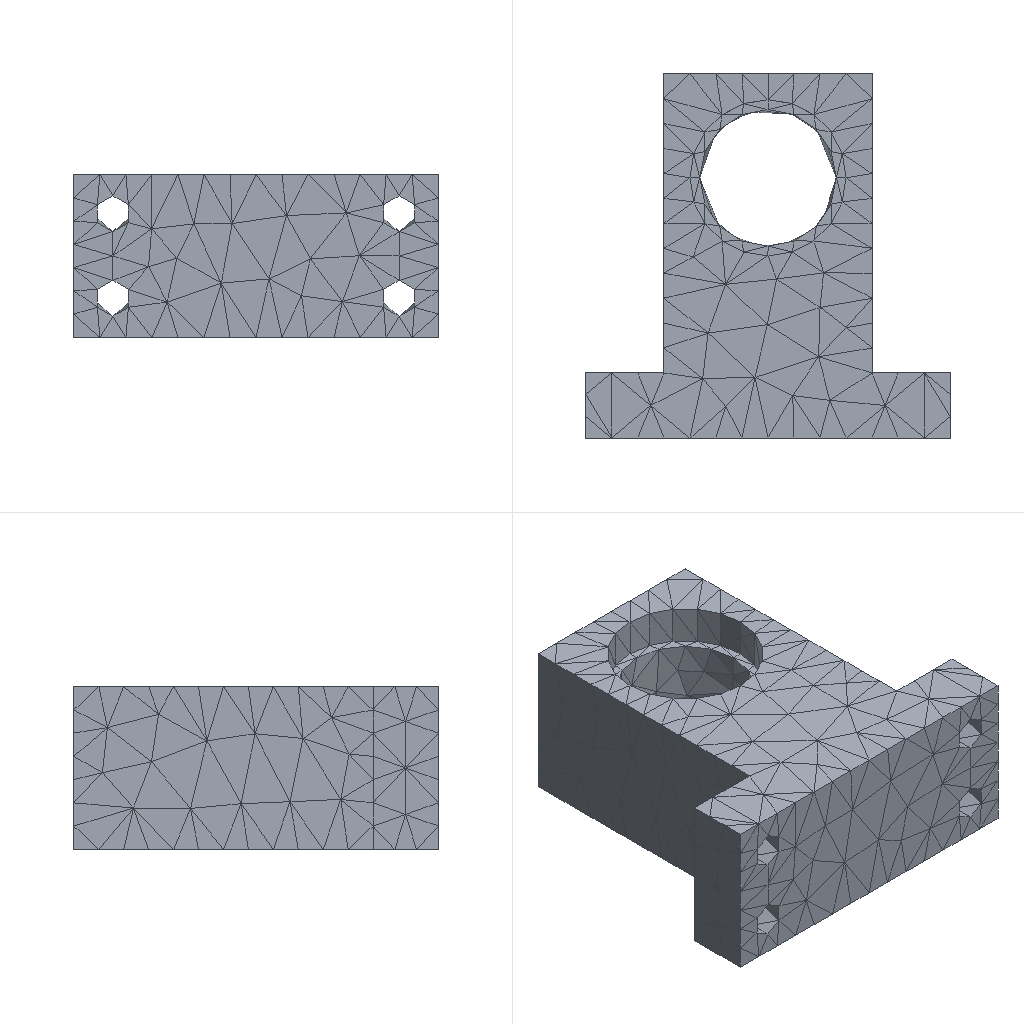Simulation study | ansys mapdl
Set-up summary:
category,name,step,type,value,unit,region
solver,ansys_mapdl
solver,version,,,22.1
units,MPA,,stated
analysis,deck,,static,static
load_step,requested,,,1
analysis,nlgeom,,,False
mesh,nodes,,,3282
mesh,elements,,,1777
element_type,ANSYS 187 (type 1),,solid,1667
element_type,ANSYS 154 (type 2),,surface,110
load,load commands in deck,,count,3
bc,support commands in deck,,count,1
named_set,_FIXEDSU,,component
material,1,,in results
check,setup vs results,,match,110 surface effect element(s) are not in the reader's mesh and were not compared
Ansys APDL input file, long lists of numbers shortened:
/batch
/config,noeldb,1     ! force off writing results to database
*get,_wallstrt,active,,time,wall
! ANSYS input file written by Workbench version 2022 R1
! File used for geometry attach: [REDACTED]
/title,wbnew--____ (A5)
! ****** Begin Custom Load Command Snippet ******
/COM, ACT Extensions:
/COM,     LSDYNA, 2021.1
/COM,
! ****** End   Custom Load Command Snippet ******
*DIM,_wb_ProjectScratch_dir,string,248
_wb_ProjectScratch_dir(1) = 'C:\Users\Administrator\AppData\Local\Temp\WB_Administrator_78380_2\_ProjectScratch\Scr73FA\'
*DIM,_wb_SolverFiles_dir,string,248
_wb_SolverFiles_dir(1) = 'C:\Users\Administrator\AppData\Local\Temp\WB_Administrator_78380_2\wbnew_files\dp0\SYS\MECH\'
*DIM,_wb_userfiles_dir,string,248
_wb_userfiles_dir(1) = 'C:\Users\Administrator\AppData\Local\Temp\WB_Administrator_78380_2\wbnew_files\user_files\'
/com,--- Data in consistent NMM units. See Solving Units in the help system for more information.
/units,MPA
/nopr
/wb,file,start              !  signify a WB generated input file
/prep7
! Turn off shape checking because checks already performed inside WB mesher.
! See help system for more information.
SHPP,OFF,,NOWARN
/nolist
etcon,set             ! allow ANSYS to choose best KEYOP's for 180x elements, resets any applicable keyopt to MAPDL defaults
/com,*********** Nodes for the whole assembly ***********
nblock,3,,3610
(1i9,3e20.9e3)
        1    -2.200000000E+01    -3.000000000E+01    -9.250000000E+00
! (3281 more lines like these left out)
-1
/wb,elem,start            !  set before creation of elements
/com,*********** Elements for Body 1 "___-FreeParts|____1" ***********
et,1,187
eblock,19,solid,,1667
(19i9)
        1        1        1        1        0        0        0        0       10        0        1      103      563      422      504     1254     2831     1248     1250
! (3333 more lines like these left out)
-1
/wb,elem,end               !  done creating elements
/com,*********** Send User Defined Coordinate System(s) ***********
csys,0
toffst,273.15,  ! Temperature offset from absolute zero
/com,*********** Set Reference Temperature ***********
tref,22.
/wb,mat,start              !  starting to send materials
/com,*********** Send Materials ***********
Temperature = 'TEMP' ! Temperature
MP,DENS,1,7.85e-09,	! tonne mm^-3
MP,ALPX,1,1.2e-05,	! C^-1
MP,C,1,434000000,	! mm^2 s^-2 C^-1
MP,KXX,1,60.5,	! tonne mm s^-3 C^-1
MP,RSVX,1,0.00017,	! ohm mm
MP,EX,1,200000,	! tonne s^-2 mm^-1
MP,NUXY,1,0.3,
MP,MURX,1,10000,
/wb,mat,end                !  done sending materials
!************************* Model Summary ********************
!___-FreeParts|____1,	structural steel,	matid,	1
!************************* End Model Summary ********************
! get the diagonal of the bounding box. Needed later for other things
*get,_xmin,node,,mnloc,x
*get,_ymin,node,,mnloc,y
*get,_zmin,node,,mnloc,z
*get,_xmax,node,,mxloc,x
*get,_ymax,node,,mxloc,y
*get,_zmax,node,,mxloc,z
_ASMDIAG=(_xmax-_xmin)*(_xmax-_xmin)+(_ymax-_ymin)*(_ymax-_ymin)+(_zmax-_zmin)*(_zmax-_zmin)
_ASMDIAG=SQRT(_ASMDIAG)
/wb,contact,start          !  starting to send contact
/wb,contact,end            !  done creating contacts
/golist
/wb,load,start             !  starting to send loads
/com,*********** Fixed Supports ***********
CMBLOCK,_FIXEDSU,NODE,      240
(8i10)
         1         2         3         4         5         6         7         8
! (29 more lines like these left out)
cmsel,s,_FIXEDSU
d,all,all
nsel,all
/com,*********** Define Force Using Surface Effect Elements ***********
local,12,0,0.,0.,0.,0.,0.,0.
csys,0
et,2,154
eblock,10,,,110
(15i9)
     2638        2        2        2       12      182      219      190      190     1658     1690      190     1657
! (109 more lines like these left out)
-1
esel,s,type,,2
keyop,2,2,1                ! Apply load in local coordinate system
keyop,2,7,1                ! Use original area so load is constant in large deformation
esel,all
/gst,on,on
fini
*get,_numnode,node,0,count
*get,_numelem,elem,0,count
*get, _MAXELEMNUM, elem, 0, NUM, MAX
*get, _MAXNODENUM, node, 0, NUM, MAX
*get, _MAXELEMTYPE, etyp, 0, NUM, MAX
*get, _MAXREALCONST, real, 0, NUM, MAX
/go
/wb,load,end               !  done creating loads
/com,--- Number of total nodes = %_numnode%
/com,--- Number of contact elements = 110
/com,--- Number of spring elements = 0
/com,--- Number of bearing elements = 0
/com,--- Number of solid elements = 1667
/com,--- Number of condensed parts = 0
/com,--- Number of total elements = %_numelem%
*get,_wallbsol,active,,time,wall
/com,****************************************************************************
/com,*************************    SOLUTION       ********************************
/com,****************************************************************************
/solu
antype,0                   ! static analysis
_thickRatio=  1     ! Ratio of thick parts in the model
eqsl,pcg,1e-8,,,,,,1
cntr,print,1               ! print out contact info and also make no initial contact an error
dmpoption,emat,no             ! Don't combine emat file for DANSYS
dmpoption,esav,no             ! Don't combine esav file for DANSYS
nldiag,cont,iter           ! print out contact info each equilibrium iteration
rescontrol,,none                 ! Do not keep any restart files
/com,****************************************************
/com,******************* SOLVE FOR LS 1 OF 1 ****************
esel,s,type,,2
nsle
sfe,all,1,pres,1,0.
sfe,all,2,pres,1,0.
sfe,all,3,pres,1,-0.3165
nsel,all
esel,all
/nopr
/gopr
nsub,1,1,1
time,1.
outres,erase
outres,all,none
outres,nsol,all,
outres,rsol,all
outres,eangl,all
outres,etmp,all
outres,veng,all
outres,strs,all,
outres,epel,all,
outres,eppl,all,
outres,cont,all,
! *********** WB SOLVE COMMAND ***********
! check interactive state
*get,ANSINTER_,active,,int
*if,ANSINTER_,ne,0,then
/eof
*endif
solve
/com *************** Write FE CONNECTORS *********
CEWRITE,file,ce,,INTE
/com,****************************************************
/com,*************** FINISHED SOLVE FOR LS 1 *************
*get,_wallasol,active,,time,wall
/nopr
*get,_numnode,node,0,count
*get,_numelem,elem,0,count
*get, _MAXELEMNUM, elem, 0, NUM, MAX
*get, _MAXNODENUM, node, 0, NUM, MAX,,,INTERNAL
*get, _MAXELEMTYPE, etyp, 0, NUM, MAX
*get, _MAXREALCONST, real, 0, NUM, MAX
/gopr
*get,_PCGITER,active,,solu,cgiter
/post1
xmlo,ENCODING,ISO-8859-1
xmlo,parm
/xml,parm,xml
fini
/gopr
*get,_walldone,active,,time,wall
_preptime=(_wallbsol-_wallstrt)*3600
_solvtime=(_wallasol-_wallbsol)*3600
_posttime=(_walldone-_wallasol)*3600
_totaltim=(_walldone-_wallstrt)*3600
*get,_dlbratio,active,0,solu,dlbr
*get,_combtime,active,0,solu,comb
*get,_ssmode,active,0,solu,ssmm
*get,_ndofs,active,0,solu,ndof
*get,_sol_end_time,active,0,set,time
*if,_sol_end_time,eq,1.,then
/fclean				!clean distributed files
*endif
/com,--- Total number of nodes = %_numnode%
/com,--- Total number of elements = %_numelem%
/com,--- Element load balance ratio = %_dlbratio%
/com,--- Time to combine distributed files = %_combtime%
/com,--- Sparse memory mode = %_ssmode%
/com,--- Number of DOF = %_ndofs%
/wb,file,end               ! done with WB generated input
Results summary:
result,analysis,,,static
result,last_loadstep,,,1
result,primary field,,,displacement
result,reaction total,1,FX,0.0,N
result,reaction total,1,FY,1e-06,N
result,reaction total,1,FZ,500,N
result,mass,,,0.000314,"NMM: mm, ton, N, s, mV, mA, degC"